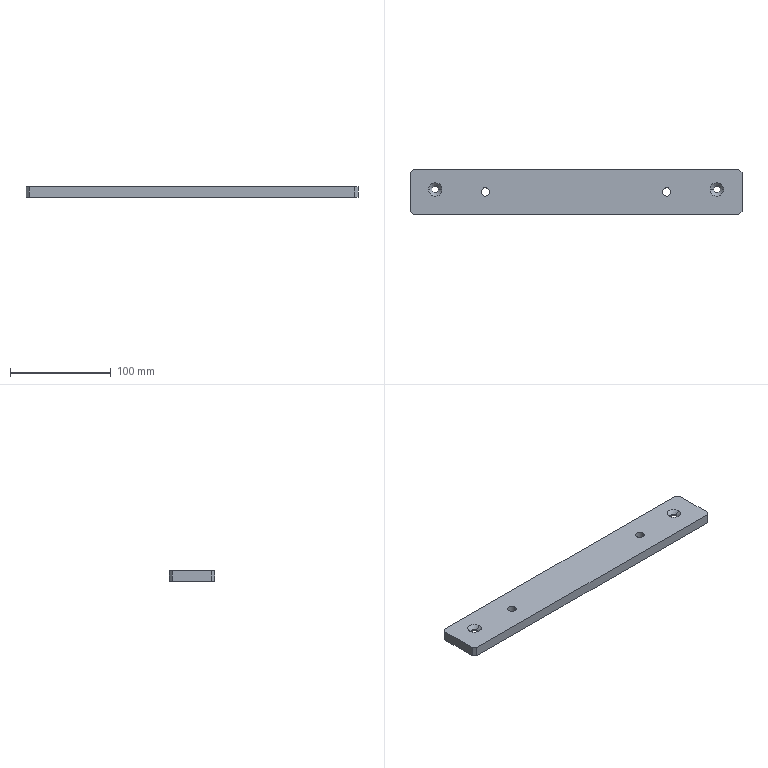Part | STEP file | 1 solid | 28 faces | box 330 x 45 x 10 mm | volume 141601 mm3 | cylinder 12 | plane 12 | cone 4 | commonest cylinder face diameters 6.6 x4 8.5 x4 25 x4